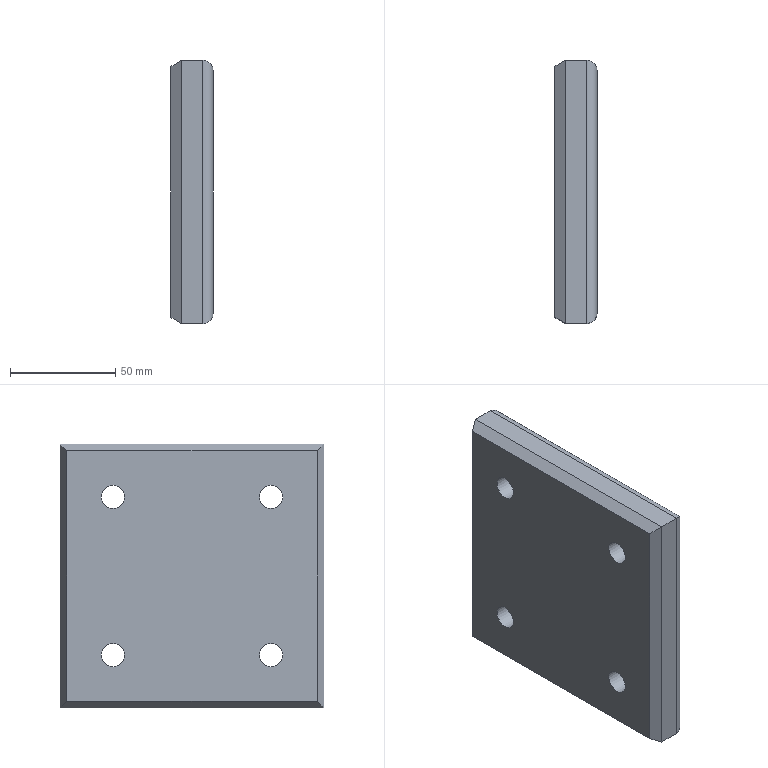Part | NX | features solid 2 | 1 solid | 30 faces | box 20 x 125 x 125 mm | volume 291132 mm3 | plane 14 | cylinder 12 | torus 4 | commonest cylinder face diameters 10 x4 11 x4 17.5 x4
STEP:
#1=CARTESIAN_POINT('',(525.,-390.,-50.));
#2=VERTEX_POINT('',#1);
#3=CARTESIAN_POINT('',(515.,-390.,-50.));
#4=VERTEX_POINT('',#3);
#5=CARTESIAN_POINT('',(530.,-390.,-50.));
#6=DIRECTION('',(-1.,0.,0.));
#7=VECTOR('',#6,1000.);
#8=LINE('',#5,#7);
#9=EDGE_CURVE('',#2,#4,#8,.T.);
#10=ORIENTED_EDGE('',*,*,#9,.F.);
#11=CARTESIAN_POINT('',(525.,-265.,-50.));
#12=VERTEX_POINT('',#11);
#13=CARTESIAN_POINT('',(525.,-290.,-50.));
#14=DIRECTION('',(0.,-1.,0.));
#15=VECTOR('',#14,1000.);
#16=LINE('',#13,#15);
#17=EDGE_CURVE('',#12,#2,#16,.T.);
#18=ORIENTED_EDGE('',*,*,#17,.F.);
#19=CARTESIAN_POINT('',(515.,-265.,-50.));
#20=VERTEX_POINT('',#19);
#21=CARTESIAN_POINT('',(530.,-265.,-50.));
#22=DIRECTION('',(-1.,0.,0.));
#23=VECTOR('',#22,1000.);
#24=LINE('',#21,#23);
#25=EDGE_CURVE('',#12,#20,#24,.T.);
#26=ORIENTED_EDGE('',*,*,#25,.T.);
#27=CARTESIAN_POINT('',(515.,-265.,-50.));
#28=DIRECTION('',(0.,1.,0.));
#29=VECTOR('',#28,1000.);
#30=LINE('',#27,#29);
#31=EDGE_CURVE('',#4,#20,#30,.T.);
#32=ORIENTED_EDGE('',*,*,#31,.F.);
#33=EDGE_LOOP('',(#10,#18,#26,#32));
#34=FACE_BOUND('',#33,.T.);
#35=CARTESIAN_POINT('',(530.,-290.,-50.));
#36=DIRECTION('',(0.,0.,1.));
#37=DIRECTION('',(-1.,0.,0.));
#38=AXIS2_PLACEMENT_3D('',#35,#36,#37);
#39=PLANE('',#38);
#40=ADVANCED_FACE('',(#34),#39,.T.);
#41=ORIENTED_EDGE('',*,*,#25,.F.);
#42=CARTESIAN_POINT('',(525.,-265.,-175.));
#43=VERTEX_POINT('',#42);
#44=CARTESIAN_POINT('',(525.,-265.,-200.));
#45=DIRECTION('',(0.,0.,1.));
#46=VECTOR('',#45,1000.);
#47=LINE('',#44,#46);
#48=EDGE_CURVE('',#43,#12,#47,.T.);
#49=ORIENTED_EDGE('',*,*,#48,.F.);
#50=CARTESIAN_POINT('',(515.,-265.,-175.));
#51=VERTEX_POINT('',#50);
#52=CARTESIAN_POINT('',(530.,-265.,-175.));
#53=DIRECTION('',(-1.,0.,0.));
#54=VECTOR('',#53,1000.);
#55=LINE('',#52,#54);
#56=EDGE_CURVE('',#43,#51,#55,.T.);
#57=ORIENTED_EDGE('',*,*,#56,.T.);
#58=CARTESIAN_POINT('',(515.,-265.,-175.));
#59=DIRECTION('',(0.,0.,-1.));
#60=VECTOR('',#59,1000.);
#61=LINE('',#58,#60);
#62=EDGE_CURVE('',#20,#51,#61,.T.);
#63=ORIENTED_EDGE('',*,*,#62,.F.);
#64=EDGE_LOOP('',(#41,#49,#57,#63));
#65=FACE_BOUND('',#64,.T.);
#66=CARTESIAN_POINT('',(530.,-265.,-200.));
#67=DIRECTION('',(0.,1.,0.));
#68=DIRECTION('',(0.,0.,1.));
#69=AXIS2_PLACEMENT_3D('',#66,#67,#68);
#70=PLANE('',#69);
#71=ADVANCED_FACE('',(#65),#70,.T.);
#72=ORIENTED_EDGE('',*,*,#56,.F.);
#73=CARTESIAN_POINT('',(525.,-390.,-175.));
#74=VERTEX_POINT('',#73);
#75=CARTESIAN_POINT('',(525.,-265.,-175.));
#76=DIRECTION('',(0.,-1.,0.));
#77=VECTOR('',#76,1000.);
#78=LINE('',#75,#77);
#79=EDGE_CURVE('',#74,#43,#78,.F.);
#80=ORIENTED_EDGE('',*,*,#79,.F.);
#81=CARTESIAN_POINT('',(515.,-390.,-175.));
#82=VERTEX_POINT('',#81);
#83=CARTESIAN_POINT('',(530.,-390.,-175.));
#84=DIRECTION('',(-1.,0.,0.));
#85=VECTOR('',#84,1000.);
#86=LINE('',#83,#85);
#87=EDGE_CURVE('',#74,#82,#86,.T.);
#88=ORIENTED_EDGE('',*,*,#87,.T.);
#89=CARTESIAN_POINT('',(515.,-290.,-175.));
#90=DIRECTION('',(0.,-1.,0.));
#91=VECTOR('',#90,1000.);
#92=LINE('',#89,#91);
#93=EDGE_CURVE('',#51,#82,#92,.T.);
#94=ORIENTED_EDGE('',*,*,#93,.F.);
#95=EDGE_LOOP('',(#72,#80,#88,#94));
#96=FACE_BOUND('',#95,.T.);
#97=CARTESIAN_POINT('',(530.,-290.,-175.));
#98=DIRECTION('',(0.,0.,1.));
#99=DIRECTION('',(-1.,0.,0.));
#100=AXIS2_PLACEMENT_3D('',#97,#98,#99);
#101=PLANE('',#100);
#102=ADVANCED_FACE('',(#96),#101,.F.);
#103=ORIENTED_EDGE('',*,*,#87,.F.);
#104=CARTESIAN_POINT('',(525.,-390.,-175.));
#105=DIRECTION('',(0.,0.,1.));
#106=VECTOR('',#105,1000.);
#107=LINE('',#104,#106);
#108=EDGE_CURVE('',#2,#74,#107,.F.);
#109=ORIENTED_EDGE('',*,*,#108,.F.);
#110=ORIENTED_EDGE('',*,*,#9,.T.);
#111=CARTESIAN_POINT('',(515.,-390.,-200.));
#112=DIRECTION('',(0.,0.,1.));
#113=VECTOR('',#112,1000.);
#114=LINE('',#111,#113);
#115=EDGE_CURVE('',#82,#4,#114,.T.);
#116=ORIENTED_EDGE('',*,*,#115,.F.);
#117=EDGE_LOOP('',(#103,#109,#110,#116));
#118=FACE_BOUND('',#117,.T.);
#119=CARTESIAN_POINT('',(530.,-390.,-200.));
#120=DIRECTION('',(0.,1.,0.));
#121=DIRECTION('',(0.,0.,1.));
#122=AXIS2_PLACEMENT_3D('',#119,#120,#121);
#123=PLANE('',#122);
#124=ADVANCED_FACE('',(#118),#123,.F.);
#125=CARTESIAN_POINT('',(530.,-290.,-138.25));
#126=VERTEX_POINT('',#125);
#127=CARTESIAN_POINT('',(530.,-290.,-150.));
#128=DIRECTION('',(-1.,0.,0.));
#129=DIRECTION('',(0.,0.,1.));
#130=AXIS2_PLACEMENT_3D('',#127,#128,#129);
#131=CIRCLE('',#130,11.75);
#132=EDGE_CURVE('',#126,#126,#131,.F.);
#133=ORIENTED_EDGE('',*,*,#132,.F.);
#134=EDGE_LOOP('',(#133));
#135=FACE_BOUND('',#134,.T.);
#136=CARTESIAN_POINT('',(530.,-365.,-138.25));
#137=VERTEX_POINT('',#136);
#138=CARTESIAN_POINT('',(530.,-365.,-150.));
#139=DIRECTION('',(-1.,0.,0.));
#140=DIRECTION('',(0.,0.,1.));
#141=AXIS2_PLACEMENT_3D('',#138,#139,#140);
#142=CIRCLE('',#141,11.75);
#143=EDGE_CURVE('',#137,#137,#142,.F.);
#144=ORIENTED_EDGE('',*,*,#143,.F.);
#145=EDGE_LOOP('',(#144));
#146=FACE_BOUND('',#145,.T.);
#147=CARTESIAN_POINT('',(530.,-365.,-63.25));
#148=VERTEX_POINT('',#147);
#149=CARTESIAN_POINT('',(530.,-365.,-75.));
#150=DIRECTION('',(-1.,0.,0.));
#151=DIRECTION('',(0.,0.,1.));
#152=AXIS2_PLACEMENT_3D('',#149,#150,#151);
#153=CIRCLE('',#152,11.75);
#154=EDGE_CURVE('',#148,#148,#153,.F.);
#155=ORIENTED_EDGE('',*,*,#154,.F.);
#156=EDGE_LOOP('',(#155));
#157=FACE_BOUND('',#156,.T.);
#158=CARTESIAN_POINT('',(530.,-290.,-63.25));
#159=VERTEX_POINT('',#158);
#160=CARTESIAN_POINT('',(530.,-290.,-75.));
#161=DIRECTION('',(-1.,0.,0.));
#162=DIRECTION('',(0.,0.,1.));
#163=AXIS2_PLACEMENT_3D('',#160,#161,#162);
#164=CIRCLE('',#163,11.75);
#165=EDGE_CURVE('',#159,#159,#164,.F.);
#166=ORIENTED_EDGE('',*,*,#165,.F.);
#167=EDGE_LOOP('',(#166));
#168=FACE_BOUND('',#167,.T.);
#169=CARTESIAN_POINT('',(530.,-385.,-55.));
#170=VERTEX_POINT('',#169);
#171=CARTESIAN_POINT('',(530.,-270.,-55.));
#172=VERTEX_POINT('',#171);
#173=CARTESIAN_POINT('',(530.,-290.,-55.));
#174=DIRECTION('',(0.,-1.,0.));
#175=VECTOR('',#174,1000.);
#176=LINE('',#173,#175);
#177=EDGE_CURVE('',#170,#172,#176,.F.);
#178=ORIENTED_EDGE('',*,*,#177,.F.);
#179=CARTESIAN_POINT('',(530.,-385.,-170.));
#180=VERTEX_POINT('',#179);
#181=CARTESIAN_POINT('',(530.,-385.,-50.));
#182=DIRECTION('',(0.,0.,1.));
#183=VECTOR('',#182,1000.);
#184=LINE('',#181,#183);
#185=EDGE_CURVE('',#180,#170,#184,.T.);
#186=ORIENTED_EDGE('',*,*,#185,.F.);
#187=CARTESIAN_POINT('',(530.,-270.,-170.));
#188=VERTEX_POINT('',#187);
#189=CARTESIAN_POINT('',(530.,-390.,-170.));
#190=DIRECTION('',(0.,-1.,0.));
#191=VECTOR('',#190,1000.);
#192=LINE('',#189,#191);
#193=EDGE_CURVE('',#188,#180,#192,.T.);
#194=ORIENTED_EDGE('',*,*,#193,.F.);
#195=CARTESIAN_POINT('',(530.,-270.,-200.));
#196=DIRECTION('',(0.,0.,1.));
#197=VECTOR('',#196,1000.);
#198=LINE('',#195,#197);
#199=EDGE_CURVE('',#172,#188,#198,.F.);
#200=ORIENTED_EDGE('',*,*,#199,.F.);
#201=EDGE_LOOP('',(#178,#186,#194,#200));
#202=FACE_BOUND('',#201,.T.);
#203=CARTESIAN_POINT('',(530.,-290.,-200.));
#204=DIRECTION('',(1.,0.,0.));
#205=DIRECTION('',(0.,0.,1.));
#206=AXIS2_PLACEMENT_3D('',#203,#204,#205);
#207=PLANE('',#206);
#208=ADVANCED_FACE('',(#135,#146,#157,#168,#202),#207,.T.);
#209=CARTESIAN_POINT('',(510.,-387.,-53.));
#210=VERTEX_POINT('',#209);
#211=CARTESIAN_POINT('',(510.,-387.,-172.));
#212=VERTEX_POINT('',#211);
#213=CARTESIAN_POINT('',(510.,-387.,-200.));
#214=DIRECTION('',(0.,0.,-1.));
#215=VECTOR('',#214,1000.);
#216=LINE('',#213,#215);
#217=EDGE_CURVE('',#210,#212,#216,.T.);
#218=ORIENTED_EDGE('',*,*,#217,.F.);
#219=CARTESIAN_POINT('',(510.,-268.,-53.));
#220=VERTEX_POINT('',#219);
#221=CARTESIAN_POINT('',(510.,-390.,-53.));
#222=DIRECTION('',(0.,-1.,0.));
#223=VECTOR('',#222,1000.);
#224=LINE('',#221,#223);
#225=EDGE_CURVE('',#220,#210,#224,.T.);
#226=ORIENTED_EDGE('',*,*,#225,.F.);
#227=CARTESIAN_POINT('',(510.,-268.,-172.));
#228=VERTEX_POINT('',#227);
#229=CARTESIAN_POINT('',(510.,-268.,-50.));
#230=DIRECTION('',(0.,0.,1.));
#231=VECTOR('',#230,1000.);
#232=LINE('',#229,#231);
#233=EDGE_CURVE('',#228,#220,#232,.T.);
#234=ORIENTED_EDGE('',*,*,#233,.F.);
#235=CARTESIAN_POINT('',(510.,-290.,-172.));
#236=DIRECTION('',(0.,1.,0.));
#237=VECTOR('',#236,1000.);
#238=LINE('',#235,#237);
#239=EDGE_CURVE('',#212,#228,#238,.T.);
#240=ORIENTED_EDGE('',*,*,#239,.F.);
#241=EDGE_LOOP('',(#218,#226,#234,#240));
#242=FACE_BOUND('',#241,.T.);
#243=CARTESIAN_POINT('',(510.,-365.,-144.5));
#244=VERTEX_POINT('',#243);
#245=CARTESIAN_POINT('',(510.,-365.,-150.));
#246=DIRECTION('',(-1.,0.,0.));
#247=DIRECTION('',(0.,0.,1.));
#248=AXIS2_PLACEMENT_3D('',#245,#246,#247);
#249=CIRCLE('',#248,5.5);
#250=EDGE_CURVE('',#244,#244,#249,.T.);
#251=ORIENTED_EDGE('',*,*,#250,.F.);
#252=EDGE_LOOP('',(#251));
#253=FACE_BOUND('',#252,.T.);
#254=CARTESIAN_POINT('',(510.,-290.,-144.5));
#255=VERTEX_POINT('',#254);
#256=CARTESIAN_POINT('',(510.,-290.,-150.));
#257=DIRECTION('',(-1.,0.,0.));
#258=DIRECTION('',(0.,0.,1.));
#259=AXIS2_PLACEMENT_3D('',#256,#257,#258);
#260=CIRCLE('',#259,5.5);
#261=EDGE_CURVE('',#255,#255,#260,.T.);
#262=ORIENTED_EDGE('',*,*,#261,.F.);
#263=EDGE_LOOP('',(#262));
#264=FACE_BOUND('',#263,.T.);
#265=CARTESIAN_POINT('',(510.,-365.,-69.5));
#266=VERTEX_POINT('',#265);
#267=CARTESIAN_POINT('',(510.,-365.,-75.));
#268=DIRECTION('',(-1.,0.,0.));
#269=DIRECTION('',(0.,0.,1.));
#270=AXIS2_PLACEMENT_3D('',#267,#268,#269);
#271=CIRCLE('',#270,5.5);
#272=EDGE_CURVE('',#266,#266,#271,.T.);
#273=ORIENTED_EDGE('',*,*,#272,.F.);
#274=EDGE_LOOP('',(#273));
#275=FACE_BOUND('',#274,.T.);
#276=CARTESIAN_POINT('',(510.,-290.,-69.5));
#277=VERTEX_POINT('',#276);
#278=CARTESIAN_POINT('',(510.,-290.,-75.));
#279=DIRECTION('',(-1.,0.,0.));
#280=DIRECTION('',(0.,0.,1.));
#281=AXIS2_PLACEMENT_3D('',#278,#279,#280);
#282=CIRCLE('',#281,5.5);
#283=EDGE_CURVE('',#277,#277,#282,.T.);
#284=ORIENTED_EDGE('',*,*,#283,.F.);
#285=EDGE_LOOP('',(#284));
#286=FACE_BOUND('',#285,.T.);
#287=CARTESIAN_POINT('',(510.,-290.,-200.));
#288=DIRECTION('',(1.,0.,0.));
#289=DIRECTION('',(0.,0.,1.));
#290=AXIS2_PLACEMENT_3D('',#287,#288,#289);
#291=PLANE('',#290);
#292=ADVANCED_FACE('',(#242,#253,#264,#275,#286),#291,.F.);
#293=CARTESIAN_POINT('',(518.,-290.,-80.5));
#294=VERTEX_POINT('',#293);
#295=CARTESIAN_POINT('',(518.,-290.,-75.));
#296=DIRECTION('',(1.,0.,0.));
#297=DIRECTION('',(0.,0.,-1.));
#298=AXIS2_PLACEMENT_3D('',#295,#296,#297);
#299=CIRCLE('',#298,5.5);
#300=EDGE_CURVE('',#294,#294,#299,.T.);
#301=ORIENTED_EDGE('',*,*,#300,.T.);
#302=EDGE_LOOP('',(#301));
#303=FACE_BOUND('',#302,.T.);
#304=ORIENTED_EDGE('',*,*,#283,.T.);
#305=EDGE_LOOP('',(#304));
#306=FACE_BOUND('',#305,.T.);
#307=CARTESIAN_POINT('',(480.,-290.,-75.));
#308=DIRECTION('',(-1.,0.,0.));
#309=DIRECTION('',(0.,0.,-1.));
#310=AXIS2_PLACEMENT_3D('',#307,#308,#309);
#311=CYLINDRICAL_SURFACE('',#310,5.5);
#312=ADVANCED_FACE('',(#303,#306),#311,.F.);
#313=ORIENTED_EDGE('',*,*,#300,.F.);
#314=EDGE_LOOP('',(#313));
#315=FACE_BOUND('',#314,.T.);
#316=CARTESIAN_POINT('',(518.,-290.,-83.75));
#317=VERTEX_POINT('',#316);
#318=CARTESIAN_POINT('',(518.,-290.,-75.));
#319=DIRECTION('',(1.,0.,0.));
#320=DIRECTION('',(0.,0.,-1.));
#321=AXIS2_PLACEMENT_3D('',#318,#319,#320);
#322=CIRCLE('',#321,8.75);
#323=EDGE_CURVE('',#317,#317,#322,.T.);
#324=ORIENTED_EDGE('',*,*,#323,.T.);
#325=EDGE_LOOP('',(#324));
#326=FACE_BOUND('',#325,.T.);
#327=CARTESIAN_POINT('',(518.,-290.,-75.));
#328=DIRECTION('',(-1.,0.,0.));
#329=DIRECTION('',(0.,0.,-1.));
#330=AXIS2_PLACEMENT_3D('',#327,#328,#329);
#331=PLANE('',#330);
#332=ADVANCED_FACE('',(#315,#326),#331,.F.);
#333=CARTESIAN_POINT('',(527.,-290.,-66.25));
#334=VERTEX_POINT('',#333);
#335=CARTESIAN_POINT('',(527.,-290.,-75.));
#336=DIRECTION('',(-1.,0.,0.));
#337=DIRECTION('',(0.,0.,1.));
#338=AXIS2_PLACEMENT_3D('',#335,#336,#337);
#339=CIRCLE('',#338,8.75);
#340=EDGE_CURVE('',#334,#334,#339,.T.);
#341=ORIENTED_EDGE('',*,*,#340,.F.);
#342=EDGE_LOOP('',(#341));
#343=FACE_BOUND('',#342,.T.);
#344=ORIENTED_EDGE('',*,*,#323,.F.);
#345=EDGE_LOOP('',(#344));
#346=FACE_BOUND('',#345,.T.);
#347=CARTESIAN_POINT('',(530.,-290.,-75.));
#348=DIRECTION('',(-1.,0.,0.));
#349=DIRECTION('',(0.,0.,-1.));
#350=AXIS2_PLACEMENT_3D('',#347,#348,#349);
#351=CYLINDRICAL_SURFACE('',#350,8.75);
#352=ADVANCED_FACE('',(#343,#346),#351,.F.);
#353=CARTESIAN_POINT('',(518.,-365.,-80.5));
#354=VERTEX_POINT('',#353);
#355=CARTESIAN_POINT('',(518.,-365.,-75.));
#356=DIRECTION('',(1.,0.,0.));
#357=DIRECTION('',(0.,0.,-1.));
#358=AXIS2_PLACEMENT_3D('',#355,#356,#357);
#359=CIRCLE('',#358,5.5);
#360=EDGE_CURVE('',#354,#354,#359,.T.);
#361=ORIENTED_EDGE('',*,*,#360,.T.);
#362=EDGE_LOOP('',(#361));
#363=FACE_BOUND('',#362,.T.);
#364=ORIENTED_EDGE('',*,*,#272,.T.);
#365=EDGE_LOOP('',(#364));
#366=FACE_BOUND('',#365,.T.);
#367=CARTESIAN_POINT('',(480.,-365.,-75.));
#368=DIRECTION('',(-1.,0.,0.));
#369=DIRECTION('',(0.,0.,-1.));
#370=AXIS2_PLACEMENT_3D('',#367,#368,#369);
#371=CYLINDRICAL_SURFACE('',#370,5.5);
#372=ADVANCED_FACE('',(#363,#366),#371,.F.);
#373=ORIENTED_EDGE('',*,*,#360,.F.);
#374=EDGE_LOOP('',(#373));
#375=FACE_BOUND('',#374,.T.);
#376=CARTESIAN_POINT('',(518.,-365.,-83.75));
#377=VERTEX_POINT('',#376);
#378=CARTESIAN_POINT('',(518.,-365.,-75.));
#379=DIRECTION('',(1.,0.,0.));
#380=DIRECTION('',(0.,0.,-1.));
#381=AXIS2_PLACEMENT_3D('',#378,#379,#380);
#382=CIRCLE('',#381,8.75);
#383=EDGE_CURVE('',#377,#377,#382,.T.);
#384=ORIENTED_EDGE('',*,*,#383,.T.);
#385=EDGE_LOOP('',(#384));
#386=FACE_BOUND('',#385,.T.);
#387=CARTESIAN_POINT('',(518.,-365.,-75.));
#388=DIRECTION('',(-1.,0.,0.));
#389=DIRECTION('',(0.,0.,-1.));
#390=AXIS2_PLACEMENT_3D('',#387,#388,#389);
#391=PLANE('',#390);
#392=ADVANCED_FACE('',(#375,#386),#391,.F.);
#393=CARTESIAN_POINT('',(527.,-365.,-66.25));
#394=VERTEX_POINT('',#393);
#395=CARTESIAN_POINT('',(527.,-365.,-75.));
#396=DIRECTION('',(-1.,0.,0.));
#397=DIRECTION('',(0.,0.,1.));
#398=AXIS2_PLACEMENT_3D('',#395,#396,#397);
#399=CIRCLE('',#398,8.75);
#400=EDGE_CURVE('',#394,#394,#399,.T.);
#401=ORIENTED_EDGE('',*,*,#400,.F.);
#402=EDGE_LOOP('',(#401));
#403=FACE_BOUND('',#402,.T.);
#404=ORIENTED_EDGE('',*,*,#383,.F.);
#405=EDGE_LOOP('',(#404));
#406=FACE_BOUND('',#405,.T.);
#407=CARTESIAN_POINT('',(530.,-365.,-75.));
#408=DIRECTION('',(-1.,0.,0.));
#409=DIRECTION('',(0.,0.,-1.));
#410=AXIS2_PLACEMENT_3D('',#407,#408,#409);
#411=CYLINDRICAL_SURFACE('',#410,8.75);
#412=ADVANCED_FACE('',(#403,#406),#411,.F.);
#413=CARTESIAN_POINT('',(518.,-290.,-155.5));
#414=VERTEX_POINT('',#413);
#415=CARTESIAN_POINT('',(518.,-290.,-150.));
#416=DIRECTION('',(1.,0.,0.));
#417=DIRECTION('',(0.,0.,-1.));
#418=AXIS2_PLACEMENT_3D('',#415,#416,#417);
#419=CIRCLE('',#418,5.5);
#420=EDGE_CURVE('',#414,#414,#419,.T.);
#421=ORIENTED_EDGE('',*,*,#420,.T.);
#422=EDGE_LOOP('',(#421));
#423=FACE_BOUND('',#422,.T.);
#424=ORIENTED_EDGE('',*,*,#261,.T.);
#425=EDGE_LOOP('',(#424));
#426=FACE_BOUND('',#425,.T.);
#427=CARTESIAN_POINT('',(480.,-290.,-150.));
#428=DIRECTION('',(-1.,0.,0.));
#429=DIRECTION('',(0.,0.,-1.));
#430=AXIS2_PLACEMENT_3D('',#427,#428,#429);
#431=CYLINDRICAL_SURFACE('',#430,5.5);
#432=ADVANCED_FACE('',(#423,#426),#431,.F.);
#433=ORIENTED_EDGE('',*,*,#420,.F.);
#434=EDGE_LOOP('',(#433));
#435=FACE_BOUND('',#434,.T.);
#436=CARTESIAN_POINT('',(518.,-290.,-158.75));
#437=VERTEX_POINT('',#436);
#438=CARTESIAN_POINT('',(518.,-290.,-150.));
#439=DIRECTION('',(1.,0.,0.));
#440=DIRECTION('',(0.,0.,-1.));
#441=AXIS2_PLACEMENT_3D('',#438,#439,#440);
#442=CIRCLE('',#441,8.75);
#443=EDGE_CURVE('',#437,#437,#442,.T.);
#444=ORIENTED_EDGE('',*,*,#443,.T.);
#445=EDGE_LOOP('',(#444));
#446=FACE_BOUND('',#445,.T.);
#447=CARTESIAN_POINT('',(518.,-290.,-150.));
#448=DIRECTION('',(-1.,0.,0.));
#449=DIRECTION('',(0.,0.,-1.));
#450=AXIS2_PLACEMENT_3D('',#447,#448,#449);
#451=PLANE('',#450);
#452=ADVANCED_FACE('',(#435,#446),#451,.F.);
#453=CARTESIAN_POINT('',(527.,-290.,-141.25));
#454=VERTEX_POINT('',#453);
#455=CARTESIAN_POINT('',(527.,-290.,-150.));
#456=DIRECTION('',(-1.,0.,0.));
#457=DIRECTION('',(0.,0.,1.));
#458=AXIS2_PLACEMENT_3D('',#455,#456,#457);
#459=CIRCLE('',#458,8.75);
#460=EDGE_CURVE('',#454,#454,#459,.T.);
#461=ORIENTED_EDGE('',*,*,#460,.F.);
#462=EDGE_LOOP('',(#461));
#463=FACE_BOUND('',#462,.T.);
#464=ORIENTED_EDGE('',*,*,#443,.F.);
#465=EDGE_LOOP('',(#464));
#466=FACE_BOUND('',#465,.T.);
#467=CARTESIAN_POINT('',(530.,-290.,-150.));
#468=DIRECTION('',(-1.,0.,0.));
#469=DIRECTION('',(0.,0.,-1.));
#470=AXIS2_PLACEMENT_3D('',#467,#468,#469);
#471=CYLINDRICAL_SURFACE('',#470,8.75);
#472=ADVANCED_FACE('',(#463,#466),#471,.F.);
#473=CARTESIAN_POINT('',(518.,-365.,-155.5));
#474=VERTEX_POINT('',#473);
#475=CARTESIAN_POINT('',(518.,-365.,-150.));
#476=DIRECTION('',(1.,0.,0.));
#477=DIRECTION('',(0.,0.,-1.));
#478=AXIS2_PLACEMENT_3D('',#475,#476,#477);
#479=CIRCLE('',#478,5.5);
#480=EDGE_CURVE('',#474,#474,#479,.T.);
#481=ORIENTED_EDGE('',*,*,#480,.T.);
#482=EDGE_LOOP('',(#481));
#483=FACE_BOUND('',#482,.T.);
#484=ORIENTED_EDGE('',*,*,#250,.T.);
#485=EDGE_LOOP('',(#484));
#486=FACE_BOUND('',#485,.T.);
#487=CARTESIAN_POINT('',(480.,-365.,-150.));
#488=DIRECTION('',(-1.,0.,0.));
#489=DIRECTION('',(0.,0.,-1.));
#490=AXIS2_PLACEMENT_3D('',#487,#488,#489);
#491=CYLINDRICAL_SURFACE('',#490,5.5);
#492=ADVANCED_FACE('',(#483,#486),#491,.F.);
#493=ORIENTED_EDGE('',*,*,#480,.F.);
#494=EDGE_LOOP('',(#493));
#495=FACE_BOUND('',#494,.T.);
#496=CARTESIAN_POINT('',(518.,-365.,-158.75));
#497=VERTEX_POINT('',#496);
#498=CARTESIAN_POINT('',(518.,-365.,-150.));
#499=DIRECTION('',(1.,0.,0.));
#500=DIRECTION('',(0.,0.,-1.));
#501=AXIS2_PLACEMENT_3D('',#498,#499,#500);
#502=CIRCLE('',#501,8.75);
#503=EDGE_CURVE('',#497,#497,#502,.T.);
#504=ORIENTED_EDGE('',*,*,#503,.T.);
#505=EDGE_LOOP('',(#504));
#506=FACE_BOUND('',#505,.T.);
#507=CARTESIAN_POINT('',(518.,-365.,-150.));
#508=DIRECTION('',(-1.,0.,0.));
#509=DIRECTION('',(0.,0.,-1.));
#510=AXIS2_PLACEMENT_3D('',#507,#508,#509);
#511=PLANE('',#510);
#512=ADVANCED_FACE('',(#495,#506),#511,.F.);
#513=CARTESIAN_POINT('',(527.,-365.,-141.25));
#514=VERTEX_POINT('',#513);
#515=CARTESIAN_POINT('',(527.,-365.,-150.));
#516=DIRECTION('',(-1.,0.,0.));
#517=DIRECTION('',(0.,0.,1.));
#518=AXIS2_PLACEMENT_3D('',#515,#516,#517);
#519=CIRCLE('',#518,8.75);
#520=EDGE_CURVE('',#514,#514,#519,.T.);
#521=ORIENTED_EDGE('',*,*,#520,.F.);
#522=EDGE_LOOP('',(#521));
#523=FACE_BOUND('',#522,.T.);
#524=ORIENTED_EDGE('',*,*,#503,.F.);
#525=EDGE_LOOP('',(#524));
#526=FACE_BOUND('',#525,.T.);
#527=CARTESIAN_POINT('',(530.,-365.,-150.));
#528=DIRECTION('',(-1.,0.,0.));
#529=DIRECTION('',(0.,0.,-1.));
#530=AXIS2_PLACEMENT_3D('',#527,#528,#529);
#531=CYLINDRICAL_SURFACE('',#530,8.75);
#532=ADVANCED_FACE('',(#523,#526),#531,.F.);
#533=CARTESIAN_POINT('',(525.,-385.,-55.));
#534=DIRECTION('',(0.,0.7071,0.7071));
#535=DIRECTION('',(0.,-0.7071,0.7071));
#536=AXIS2_PLACEMENT_3D('',#533,#534,#535);
#537=ELLIPSE('',#536,7.071,5.);
#538=EDGE_CURVE('',#170,#2,#537,.F.);
#539=ORIENTED_EDGE('',*,*,#538,.T.);
#540=ORIENTED_EDGE('',*,*,#108,.T.);
#541=CARTESIAN_POINT('',(525.,-385.,-170.));
#542=DIRECTION('',(0.,-0.7071,0.7071));
#543=DIRECTION('',(0.,-0.7071,-0.7071));
#544=AXIS2_PLACEMENT_3D('',#541,#542,#543);
#545=ELLIPSE('',#544,7.071,5.);
#546=EDGE_CURVE('',#74,#180,#545,.T.);
#547=ORIENTED_EDGE('',*,*,#546,.T.);
#548=ORIENTED_EDGE('',*,*,#185,.T.);
#549=EDGE_LOOP('',(#539,#540,#547,#548));
#550=FACE_BOUND('',#549,.T.);
#551=CARTESIAN_POINT('',(525.,-385.,-200.));
#552=DIRECTION('',(0.,0.,-1.));
#553=DIRECTION('',(1.,0.,0.));
#554=AXIS2_PLACEMENT_3D('',#551,#552,#553);
#555=CYLINDRICAL_SURFACE('',#554,5.);
#556=ADVANCED_FACE('',(#550),#555,.T.);
#557=ORIENTED_EDGE('',*,*,#546,.F.);
#558=ORIENTED_EDGE('',*,*,#79,.T.);
#559=CARTESIAN_POINT('',(525.,-270.,-170.));
#560=DIRECTION('',(0.,-0.7071,-0.7071));
#561=DIRECTION('',(0.,0.7071,-0.7071));
#562=AXIS2_PLACEMENT_3D('',#559,#560,#561);
#563=ELLIPSE('',#562,7.071,5.);
#564=EDGE_CURVE('',#43,#188,#563,.T.);
#565=ORIENTED_EDGE('',*,*,#564,.T.);
#566=ORIENTED_EDGE('',*,*,#193,.T.);
#567=EDGE_LOOP('',(#557,#558,#565,#566));
#568=FACE_BOUND('',#567,.T.);
#569=CARTESIAN_POINT('',(525.,-290.,-170.));
#570=DIRECTION('',(0.,1.,0.));
#571=DIRECTION('',(0.,0.,1.));
#572=AXIS2_PLACEMENT_3D('',#569,#570,#571);
#573=CYLINDRICAL_SURFACE('',#572,5.);
#574=ADVANCED_FACE('',(#568),#573,.T.);
#575=ORIENTED_EDGE('',*,*,#538,.F.);
#576=ORIENTED_EDGE('',*,*,#177,.T.);
#577=CARTESIAN_POINT('',(525.,-270.,-55.));
#578=DIRECTION('',(0.,0.7071,-0.7071));
#579=DIRECTION('',(0.,-0.7071,-0.7071));
#580=AXIS2_PLACEMENT_3D('',#577,#578,#579);
#581=ELLIPSE('',#580,7.071,5.);
#582=EDGE_CURVE('',#172,#12,#581,.F.);
#583=ORIENTED_EDGE('',*,*,#582,.T.);
#584=ORIENTED_EDGE('',*,*,#17,.T.);
#585=EDGE_LOOP('',(#575,#576,#583,#584));
#586=FACE_BOUND('',#585,.T.);
#587=CARTESIAN_POINT('',(525.,-290.,-55.));
#588=DIRECTION('',(0.,-1.,0.));
#589=DIRECTION('',(0.,0.,-1.));
#590=AXIS2_PLACEMENT_3D('',#587,#588,#589);
#591=CYLINDRICAL_SURFACE('',#590,5.);
#592=ADVANCED_FACE('',(#586),#591,.T.);
#593=ORIENTED_EDGE('',*,*,#564,.F.);
#594=ORIENTED_EDGE('',*,*,#48,.T.);
#595=ORIENTED_EDGE('',*,*,#582,.F.);
#596=ORIENTED_EDGE('',*,*,#199,.T.);
#597=EDGE_LOOP('',(#593,#594,#595,#596));
#598=FACE_BOUND('',#597,.T.);
#599=CARTESIAN_POINT('',(525.,-270.,-200.));
#600=DIRECTION('',(0.,0.,1.));
#601=DIRECTION('',(-1.,0.,0.));
#602=AXIS2_PLACEMENT_3D('',#599,#600,#601);
#603=CYLINDRICAL_SURFACE('',#602,5.);
#604=ADVANCED_FACE('',(#598),#603,.T.);
#605=ORIENTED_EDGE('',*,*,#460,.T.);
#606=EDGE_LOOP('',(#605));
#607=FACE_BOUND('',#606,.T.);
#608=ORIENTED_EDGE('',*,*,#132,.T.);
#609=EDGE_LOOP('',(#608));
#610=FACE_BOUND('',#609,.T.);
#611=CARTESIAN_POINT('',(527.,-290.,-150.));
#612=DIRECTION('',(1.,0.,0.));
#613=DIRECTION('',(0.,0.,1.));
#614=AXIS2_PLACEMENT_3D('',#611,#612,#613);
#615=TOROIDAL_SURFACE('',#614,11.75,3.);
#616=ADVANCED_FACE('',(#607,#610),#615,.T.);
#617=ORIENTED_EDGE('',*,*,#520,.T.);
#618=EDGE_LOOP('',(#617));
#619=FACE_BOUND('',#618,.T.);
#620=ORIENTED_EDGE('',*,*,#143,.T.);
#621=EDGE_LOOP('',(#620));
#622=FACE_BOUND('',#621,.T.);
#623=CARTESIAN_POINT('',(527.,-365.,-150.));
#624=DIRECTION('',(1.,0.,0.));
#625=DIRECTION('',(0.,0.,1.));
#626=AXIS2_PLACEMENT_3D('',#623,#624,#625);
#627=TOROIDAL_SURFACE('',#626,11.75,3.);
#628=ADVANCED_FACE('',(#619,#622),#627,.T.);
#629=ORIENTED_EDGE('',*,*,#400,.T.);
#630=EDGE_LOOP('',(#629));
#631=FACE_BOUND('',#630,.T.);
#632=ORIENTED_EDGE('',*,*,#154,.T.);
#633=EDGE_LOOP('',(#632));
#634=FACE_BOUND('',#633,.T.);
#635=CARTESIAN_POINT('',(527.,-365.,-75.));
#636=DIRECTION('',(1.,0.,0.));
#637=DIRECTION('',(0.,0.,1.));
#638=AXIS2_PLACEMENT_3D('',#635,#636,#637);
#639=TOROIDAL_SURFACE('',#638,11.75,3.);
#640=ADVANCED_FACE('',(#631,#634),#639,.T.);
#641=ORIENTED_EDGE('',*,*,#340,.T.);
#642=EDGE_LOOP('',(#641));
#643=FACE_BOUND('',#642,.T.);
#644=ORIENTED_EDGE('',*,*,#165,.T.);
#645=EDGE_LOOP('',(#644));
#646=FACE_BOUND('',#645,.T.);
#647=CARTESIAN_POINT('',(527.,-290.,-75.));
#648=DIRECTION('',(1.,0.,0.));
#649=DIRECTION('',(0.,0.,1.));
#650=AXIS2_PLACEMENT_3D('',#647,#648,#649);
#651=TOROIDAL_SURFACE('',#650,11.75,3.);
#652=ADVANCED_FACE('',(#643,#646),#651,.T.);
#653=CARTESIAN_POINT('',(476.163,-366.698,-73.302));
#654=DIRECTION('',(0.7625,-0.4575,0.4575));
#655=VECTOR('',#654,1000.);
#656=LINE('',#653,#655);
#657=EDGE_CURVE('',#210,#4,#656,.T.);
#658=ORIENTED_EDGE('',*,*,#657,.T.);
#659=ORIENTED_EDGE('',*,*,#31,.T.);
#660=CARTESIAN_POINT('',(458.721,-298.767,-83.767));
#661=DIRECTION('',(-0.7625,-0.4575,-0.4575));
#662=VECTOR('',#661,1000.);
#663=LINE('',#660,#662);
#664=EDGE_CURVE('',#20,#220,#663,.T.);
#665=ORIENTED_EDGE('',*,*,#664,.T.);
#666=ORIENTED_EDGE('',*,*,#225,.T.);
#667=EDGE_LOOP('',(#658,#659,#665,#666));
#668=FACE_BOUND('',#667,.T.);
#669=CARTESIAN_POINT('',(510.,-290.,-53.));
#670=DIRECTION('',(-0.5145,0.,0.8575));
#671=DIRECTION('',(-0.8575,0.,-0.5145));
#672=AXIS2_PLACEMENT_3D('',#669,#670,#671);
#673=PLANE('',#672);
#674=ADVANCED_FACE('',(#668),#673,.T.);
#675=ORIENTED_EDGE('',*,*,#664,.F.);
#676=ORIENTED_EDGE('',*,*,#62,.T.);
#677=CARTESIAN_POINT('',(519.767,-262.14,-177.86));
#678=DIRECTION('',(-0.7625,-0.4575,0.4575));
#679=VECTOR('',#678,1000.);
#680=LINE('',#677,#679);
#681=EDGE_CURVE('',#51,#228,#680,.T.);
#682=ORIENTED_EDGE('',*,*,#681,.T.);
#683=ORIENTED_EDGE('',*,*,#233,.T.);
#684=EDGE_LOOP('',(#675,#676,#682,#683));
#685=FACE_BOUND('',#684,.T.);
#686=CARTESIAN_POINT('',(510.,-268.,-200.));
#687=DIRECTION('',(-0.5145,0.8575,0.));
#688=DIRECTION('',(0.8575,0.5145,0.));
#689=AXIS2_PLACEMENT_3D('',#686,#687,#688);
#690=PLANE('',#689);
#691=ADVANCED_FACE('',(#685),#690,.T.);
#692=ORIENTED_EDGE('',*,*,#657,.F.);
#693=ORIENTED_EDGE('',*,*,#217,.T.);
#694=CARTESIAN_POINT('',(523.721,-395.233,-180.233));
#695=DIRECTION('',(-0.7625,0.4575,0.4575));
#696=VECTOR('',#695,1000.);
#697=LINE('',#694,#696);
#698=EDGE_CURVE('',#212,#82,#697,.F.);
#699=ORIENTED_EDGE('',*,*,#698,.T.);
#700=ORIENTED_EDGE('',*,*,#115,.T.);
#701=EDGE_LOOP('',(#692,#693,#699,#700));
#702=FACE_BOUND('',#701,.T.);
#703=CARTESIAN_POINT('',(515.,-390.,-200.));
#704=DIRECTION('',(0.5145,0.8575,0.));
#705=DIRECTION('',(0.8575,-0.5145,0.));
#706=AXIS2_PLACEMENT_3D('',#703,#704,#705);
#707=PLANE('',#706);
#708=ADVANCED_FACE('',(#702),#707,.F.);
#709=ORIENTED_EDGE('',*,*,#681,.F.);
#710=ORIENTED_EDGE('',*,*,#93,.T.);
#711=ORIENTED_EDGE('',*,*,#698,.F.);
#712=ORIENTED_EDGE('',*,*,#239,.T.);
#713=EDGE_LOOP('',(#709,#710,#711,#712));
#714=FACE_BOUND('',#713,.T.);
#715=CARTESIAN_POINT('',(515.,-290.,-175.));
#716=DIRECTION('',(0.5145,0.,0.8575));
#717=DIRECTION('',(-0.8575,0.,0.5145));
#718=AXIS2_PLACEMENT_3D('',#715,#716,#717);
#719=PLANE('',#718);
#720=ADVANCED_FACE('',(#714),#719,.F.);
#721=CLOSED_SHELL('',(#40,#71,#102,#124,#208,#292,#312,#332,#352,#372,#392,#412,#432,#452,#472,#492,#512,#532,#556,#574,#592,#604,#616,#628,#640,#652,#674,#691,#708,#720));
#722=MANIFOLD_SOLID_BREP('',#721);
#723=(LENGTH_UNIT()NAMED_UNIT(*)SI_UNIT(.MILLI.,.METRE.));
#724=UNCERTAINTY_MEASURE_WITH_UNIT(LENGTH_MEASURE(0.00001),#723,'','');
#725=(NAMED_UNIT(*)PLANE_ANGLE_UNIT()SI_UNIT($,.RADIAN.));
#726=(NAMED_UNIT(*)SI_UNIT($,.STERADIAN.)SOLID_ANGLE_UNIT());
#727=(GEOMETRIC_REPRESENTATION_CONTEXT(3)GLOBAL_UNCERTAINTY_ASSIGNED_CONTEXT((#724))GLOBAL_UNIT_ASSIGNED_CONTEXT((#723,#725,#726))REPRESENTATION_CONTEXT('',''));
#728=ADVANCED_BREP_SHAPE_REPRESENTATION('',(#722),#727);